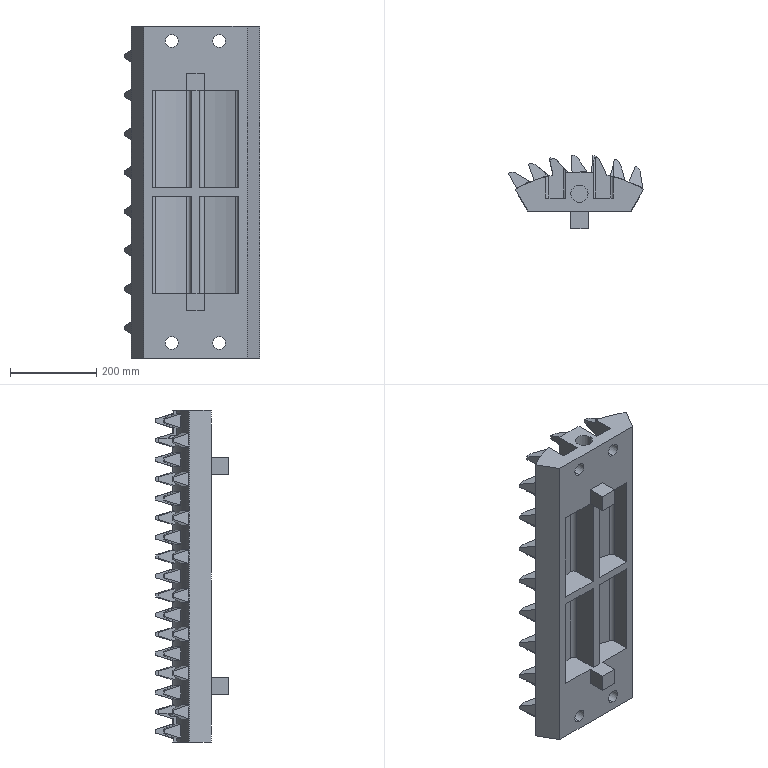Part | NX | features BREP 1, DATUM_CSYS 1, SKETCH 1 | 1 solid | 493 faces | box 313.534 x 169.472 x 770 mm | volume 12152543 mm3 | plane 401 | cylinder 92 | commonest cylinder face diameters 38 x59 10 x8 20 x8 30 x8 40 x4 550 x4